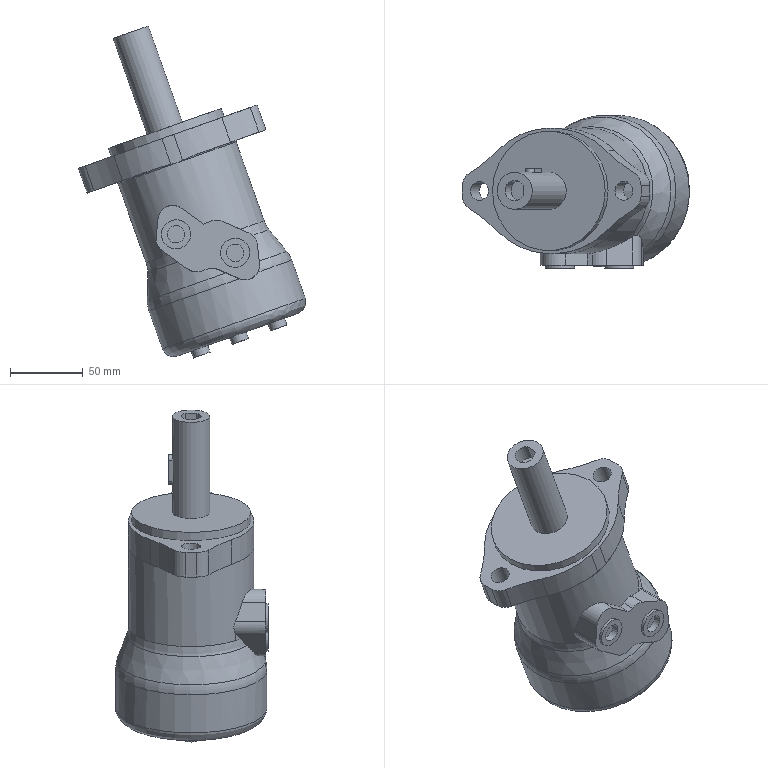Part | STEP file | MOTOR1_id422_x_t | 1 solid | 75 faces | volume 1091515 mm3 | cylinder 39 | plane 30 | other 5 | cone 1 | commonest cylinder face diameters 20 x13 12 x6 110 x4 220 x4 6 x2 13 x2